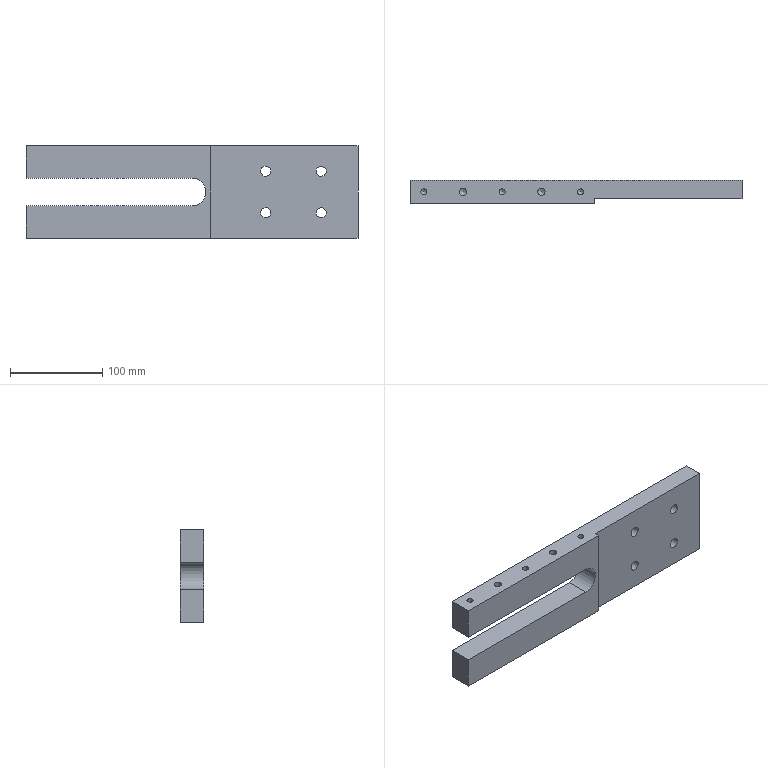Part | STEP file | SN10_002_004_PLACA | 1 solid | 40 faces | box 360 x 25 x 100 mm | volume 658656 mm3 | cylinder 17 | cone 12 | plane 11 | commonest cylinder face diameters 6.647 x8 8 x4 11 x4 30 x1